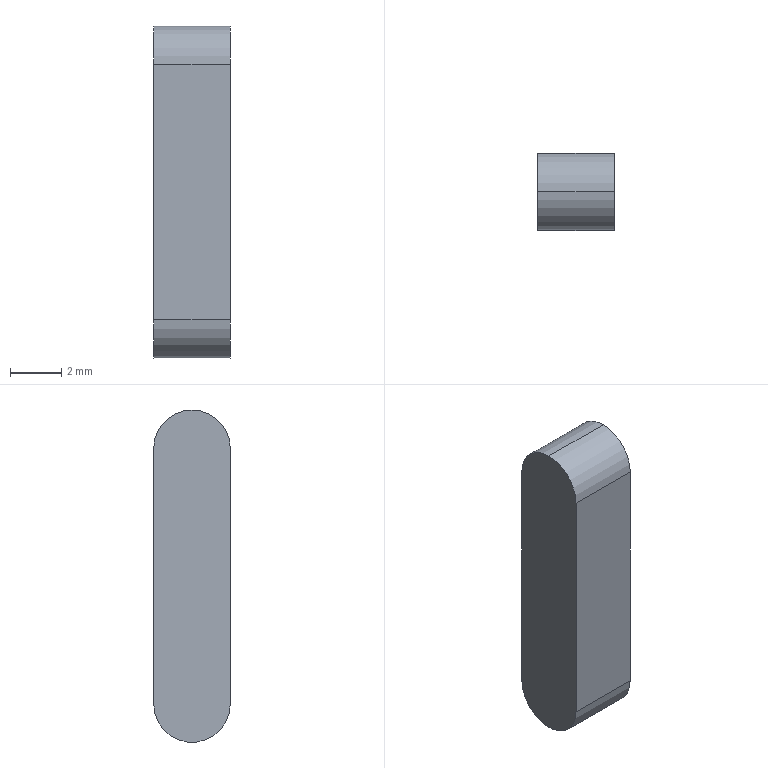Part | STEP file | 06-40 Flat key | 1 solid | 7 faces | box 3 x 3 x 13 mm | volume 111.206 mm3 | plane 4 | cylinder 3 | commonest cylinder face diameters 3 x3
STEP:
#1=CARTESIAN_POINT('',(0.,0.,0.));
#2=DIRECTION('',(0.,0.,1.));
#3=DIRECTION('',(1.,0.,0.));
#4=AXIS2_PLACEMENT_3D('',#1,#2,#3);
#5=CARTESIAN_POINT('',(3.,0.,1.5));
#6=VERTEX_POINT('',#5);
#7=CARTESIAN_POINT('',(3.,-1.5,0.));
#8=VERTEX_POINT('',#7);
#9=CARTESIAN_POINT('',(3.,0.,0.));
#10=DIRECTION('',(1.,0.,0.));
#11=DIRECTION('',(0.,0.,1.));
#12=AXIS2_PLACEMENT_3D('',#9,#10,#11);
#13=CIRCLE('',#12,1.5);
#14=CARTESIAN_POINT('',(3.,0.,0.));
#15=DIRECTION('',(-1.,0.,0.));
#16=DIRECTION('',(0.,0.,1.));
#17=AXIS2_PLACEMENT_3D('',#14,#15,#16);
#18=CYLINDRICAL_SURFACE('',#17,1.5);
#19=CARTESIAN_POINT('',(6.283,0.));
#20=DIRECTION('',(-1.,0.));
#21=VECTOR('',#20,1.);
#22=LINE('',#19,#21);
#23=(GEOMETRIC_REPRESENTATION_CONTEXT(2)PARAMETRIC_REPRESENTATION_CONTEXT()REPRESENTATION_CONTEXT('',''));
#24=DEFINITIONAL_REPRESENTATION('',(#22),#23);
#25=PCURVE('',#18,#24);
#26=CARTESIAN_POINT('',(3.,-1.5,1.578));
#27=DIRECTION('',(1.,0.,0.));
#28=DIRECTION('',(0.,0.,-1.));
#29=AXIS2_PLACEMENT_3D('',#26,#27,#28);
#30=PLANE('',#29);
#31=CARTESIAN_POINT('',(1.578,1.5));
#32=DIRECTION('',(-1.,0.));
#33=AXIS2_PLACEMENT_2D('',#31,#32);
#34=CIRCLE('',#33,1.5);
#35=(GEOMETRIC_REPRESENTATION_CONTEXT(2)PARAMETRIC_REPRESENTATION_CONTEXT()REPRESENTATION_CONTEXT('',''));
#36=DEFINITIONAL_REPRESENTATION('',(#34),#35);
#37=PCURVE('',#30,#36);
#38=SURFACE_CURVE('',#13,(#25,#37),.PCURVE_S1.);
#39=EDGE_CURVE('',#6,#8,#38,.T.);
#40=ORIENTED_EDGE('',*,*,#39,.F.);
#41=CARTESIAN_POINT('',(0.,0.,1.5));
#42=VERTEX_POINT('',#41);
#43=CARTESIAN_POINT('',(3.,0.,1.5));
#44=DIRECTION('',(-1.,0.,0.));
#45=VECTOR('',#44,1.);
#46=LINE('',#43,#45);
#47=CARTESIAN_POINT('',(6.283,0.));
#48=DIRECTION('',(0.,1.));
#49=VECTOR('',#48,1.);
#50=LINE('',#47,#49);
#51=(GEOMETRIC_REPRESENTATION_CONTEXT(2)PARAMETRIC_REPRESENTATION_CONTEXT()REPRESENTATION_CONTEXT('',''));
#52=DEFINITIONAL_REPRESENTATION('',(#50),#51);
#53=PCURVE('',#18,#52);
#54=CARTESIAN_POINT('',(3.,0.,0.));
#55=DIRECTION('',(-1.,0.,0.));
#56=DIRECTION('',(0.,0.,1.));
#57=AXIS2_PLACEMENT_3D('',#54,#55,#56);
#58=CYLINDRICAL_SURFACE('',#57,1.5);
#59=CARTESIAN_POINT('',(0.,0.));
#60=DIRECTION('',(0.,1.));
#61=VECTOR('',#60,1.);
#62=LINE('',#59,#61);
#63=(GEOMETRIC_REPRESENTATION_CONTEXT(2)PARAMETRIC_REPRESENTATION_CONTEXT()REPRESENTATION_CONTEXT('',''));
#64=DEFINITIONAL_REPRESENTATION('',(#62),#63);
#65=PCURVE('',#58,#64);
#66=SURFACE_CURVE('',#46,(#53,#65),.PCURVE_S1.);
#67=EDGE_CURVE('',#6,#42,#66,.T.);
#68=ORIENTED_EDGE('',*,*,#67,.T.);
#69=CARTESIAN_POINT('',(0.,-1.5,0.));
#70=VERTEX_POINT('',#69);
#71=CARTESIAN_POINT('',(0.,0.,0.));
#72=DIRECTION('',(-1.,0.,0.));
#73=DIRECTION('',(0.,0.,1.));
#74=AXIS2_PLACEMENT_3D('',#71,#72,#73);
#75=CIRCLE('',#74,1.5);
#76=CARTESIAN_POINT('',(0.,3.));
#77=DIRECTION('',(1.,0.));
#78=VECTOR('',#77,1.);
#79=LINE('',#76,#78);
#80=(GEOMETRIC_REPRESENTATION_CONTEXT(2)PARAMETRIC_REPRESENTATION_CONTEXT()REPRESENTATION_CONTEXT('',''));
#81=DEFINITIONAL_REPRESENTATION('',(#79),#80);
#82=PCURVE('',#18,#81);
#83=CARTESIAN_POINT('',(0.,-1.5,1.578));
#84=DIRECTION('',(1.,0.,0.));
#85=DIRECTION('',(0.,0.,-1.));
#86=AXIS2_PLACEMENT_3D('',#83,#84,#85);
#87=PLANE('',#86);
#88=CARTESIAN_POINT('',(0.078,1.5));
#89=CARTESIAN_POINT('',(0.078,4.098));
#90=CARTESIAN_POINT('',(2.328,2.799));
#91=CARTESIAN_POINT('',(4.578,1.5));
#92=CARTESIAN_POINT('',(2.328,0.201));
#93=CARTESIAN_POINT('',(0.078,-1.098));
#94=CARTESIAN_POINT('',(0.078,1.5));
#95=(BOUNDED_CURVE()B_SPLINE_CURVE(2,(#88,#89,#90,#91,#92,#93,#94),.UNSPECIFIED.,.T.,.F.)B_SPLINE_CURVE_WITH_KNOTS((1,2,2,2,2,1),(-2.094,0.,2.094,4.189,6.283,8.378),.UNSPECIFIED.)CURVE()GEOMETRIC_REPRESENTATION_ITEM()RATIONAL_B_SPLINE_CURVE((1.,0.5,1.,0.5,1.,0.5,1.))REPRESENTATION_ITEM(''));
#96=(GEOMETRIC_REPRESENTATION_CONTEXT(2)PARAMETRIC_REPRESENTATION_CONTEXT()REPRESENTATION_CONTEXT('',''));
#97=DEFINITIONAL_REPRESENTATION('',(#95),#96);
#98=PCURVE('',#87,#97);
#99=SURFACE_CURVE('',#75,(#82,#98),.PCURVE_S1.);
#100=EDGE_CURVE('',#70,#42,#99,.T.);
#101=ORIENTED_EDGE('',*,*,#100,.F.);
#102=CARTESIAN_POINT('',(1.5,-1.5,-0.000000001));
#103=DIRECTION('',(-1.,0.,0.));
#104=VECTOR('',#103,1.);
#105=LINE('',#102,#104);
#106=CARTESIAN_POINT('',(4.712,1.5));
#107=DIRECTION('',(0.,1.));
#108=VECTOR('',#107,1.);
#109=LINE('',#106,#108);
#110=(GEOMETRIC_REPRESENTATION_CONTEXT(2)PARAMETRIC_REPRESENTATION_CONTEXT()REPRESENTATION_CONTEXT('',''));
#111=DEFINITIONAL_REPRESENTATION('',(#109),#110);
#112=PCURVE('',#18,#111);
#113=CARTESIAN_POINT('',(0.,-1.5,-10.));
#114=DIRECTION('',(0.,1.,0.));
#115=DIRECTION('',(0.,0.,1.));
#116=AXIS2_PLACEMENT_3D('',#113,#114,#115);
#117=PLANE('',#116);
#118=CARTESIAN_POINT('',(10.,1.5));
#119=DIRECTION('',(0.,-1.));
#120=VECTOR('',#119,1.);
#121=LINE('',#118,#120);
#122=(GEOMETRIC_REPRESENTATION_CONTEXT(2)PARAMETRIC_REPRESENTATION_CONTEXT()REPRESENTATION_CONTEXT('',''));
#123=DEFINITIONAL_REPRESENTATION('',(#121),#122);
#124=PCURVE('',#117,#123);
#125=SURFACE_CURVE('',#105,(#112,#124),.PCURVE_S1.);
#126=EDGE_CURVE('',#8,#70,#125,.T.);
#127=ORIENTED_EDGE('',*,*,#126,.F.);
#128=EDGE_LOOP('',(#40,#68,#101,#127));
#129=FACE_BOUND('',#128,.T.);
#130=ADVANCED_FACE('',(#129),#18,.T.);
#131=ORIENTED_EDGE('',*,*,#67,.F.);
#132=CARTESIAN_POINT('',(3.,1.5,0.));
#133=VERTEX_POINT('',#132);
#134=CARTESIAN_POINT('',(3.,0.,0.));
#135=DIRECTION('',(1.,0.,0.));
#136=DIRECTION('',(0.,0.,1.));
#137=AXIS2_PLACEMENT_3D('',#134,#135,#136);
#138=CIRCLE('',#137,1.5);
#139=CARTESIAN_POINT('',(6.283,0.));
#140=DIRECTION('',(-1.,0.));
#141=VECTOR('',#140,1.);
#142=LINE('',#139,#141);
#143=(GEOMETRIC_REPRESENTATION_CONTEXT(2)PARAMETRIC_REPRESENTATION_CONTEXT()REPRESENTATION_CONTEXT('',''));
#144=DEFINITIONAL_REPRESENTATION('',(#142),#143);
#145=PCURVE('',#58,#144);
#146=CARTESIAN_POINT('',(1.578,1.5));
#147=DIRECTION('',(-1.,0.));
#148=AXIS2_PLACEMENT_2D('',#146,#147);
#149=CIRCLE('',#148,1.5);
#150=(GEOMETRIC_REPRESENTATION_CONTEXT(2)PARAMETRIC_REPRESENTATION_CONTEXT()REPRESENTATION_CONTEXT('',''));
#151=DEFINITIONAL_REPRESENTATION('',(#149),#150);
#152=PCURVE('',#30,#151);
#153=SURFACE_CURVE('',#138,(#145,#152),.PCURVE_S1.);
#154=EDGE_CURVE('',#133,#6,#153,.T.);
#155=ORIENTED_EDGE('',*,*,#154,.F.);
#156=CARTESIAN_POINT('',(0.,1.5,0.));
#157=VERTEX_POINT('',#156);
#158=CARTESIAN_POINT('',(1.5,1.5,0.));
#159=DIRECTION('',(1.,0.,0.));
#160=VECTOR('',#159,1.);
#161=LINE('',#158,#160);
#162=CARTESIAN_POINT('',(1.571,1.5));
#163=DIRECTION('',(0.,-1.));
#164=VECTOR('',#163,1.);
#165=LINE('',#162,#164);
#166=(GEOMETRIC_REPRESENTATION_CONTEXT(2)PARAMETRIC_REPRESENTATION_CONTEXT()REPRESENTATION_CONTEXT('',''));
#167=DEFINITIONAL_REPRESENTATION('',(#165),#166);
#168=PCURVE('',#58,#167);
#169=CARTESIAN_POINT('',(0.,1.5,0.));
#170=DIRECTION('',(0.,-1.,0.));
#171=DIRECTION('',(0.,0.,-1.));
#172=AXIS2_PLACEMENT_3D('',#169,#170,#171);
#173=PLANE('',#172);
#174=CARTESIAN_POINT('',(0.,1.5));
#175=DIRECTION('',(0.,1.));
#176=VECTOR('',#175,1.);
#177=LINE('',#174,#176);
#178=(GEOMETRIC_REPRESENTATION_CONTEXT(2)PARAMETRIC_REPRESENTATION_CONTEXT()REPRESENTATION_CONTEXT('',''));
#179=DEFINITIONAL_REPRESENTATION('',(#177),#178);
#180=PCURVE('',#173,#179);
#181=SURFACE_CURVE('',#161,(#168,#180),.PCURVE_S1.);
#182=EDGE_CURVE('',#157,#133,#181,.T.);
#183=ORIENTED_EDGE('',*,*,#182,.F.);
#184=CARTESIAN_POINT('',(0.,0.,0.));
#185=DIRECTION('',(-1.,0.,0.));
#186=DIRECTION('',(0.,0.,1.));
#187=AXIS2_PLACEMENT_3D('',#184,#185,#186);
#188=CIRCLE('',#187,1.5);
#189=CARTESIAN_POINT('',(0.,3.));
#190=DIRECTION('',(1.,0.));
#191=VECTOR('',#190,1.);
#192=LINE('',#189,#191);
#193=(GEOMETRIC_REPRESENTATION_CONTEXT(2)PARAMETRIC_REPRESENTATION_CONTEXT()REPRESENTATION_CONTEXT('',''));
#194=DEFINITIONAL_REPRESENTATION('',(#192),#193);
#195=PCURVE('',#58,#194);
#196=CARTESIAN_POINT('',(0.078,1.5));
#197=CARTESIAN_POINT('',(0.078,4.098));
#198=CARTESIAN_POINT('',(2.328,2.799));
#199=CARTESIAN_POINT('',(4.578,1.5));
#200=CARTESIAN_POINT('',(2.328,0.201));
#201=CARTESIAN_POINT('',(0.078,-1.098));
#202=CARTESIAN_POINT('',(0.078,1.5));
#203=(BOUNDED_CURVE()B_SPLINE_CURVE(2,(#196,#197,#198,#199,#200,#201,#202),.UNSPECIFIED.,.T.,.F.)B_SPLINE_CURVE_WITH_KNOTS((1,2,2,2,2,1),(-2.094,0.,2.094,4.189,6.283,8.378),.UNSPECIFIED.)CURVE()GEOMETRIC_REPRESENTATION_ITEM()RATIONAL_B_SPLINE_CURVE((1.,0.5,1.,0.5,1.,0.5,1.))REPRESENTATION_ITEM(''));
#204=(GEOMETRIC_REPRESENTATION_CONTEXT(2)PARAMETRIC_REPRESENTATION_CONTEXT()REPRESENTATION_CONTEXT('',''));
#205=DEFINITIONAL_REPRESENTATION('',(#203),#204);
#206=PCURVE('',#87,#205);
#207=SURFACE_CURVE('',#188,(#195,#206),.PCURVE_S1.);
#208=EDGE_CURVE('',#42,#157,#207,.T.);
#209=ORIENTED_EDGE('',*,*,#208,.F.);
#210=EDGE_LOOP('',(#131,#155,#183,#209));
#211=FACE_BOUND('',#210,.T.);
#212=ADVANCED_FACE('',(#211),#58,.T.);
#213=CARTESIAN_POINT('',(3.,-1.5,-10.));
#214=VERTEX_POINT('',#213);
#215=CARTESIAN_POINT('',(3.,1.5,-10.));
#216=VERTEX_POINT('',#215);
#217=CARTESIAN_POINT('',(3.,0.,-10.));
#218=DIRECTION('',(1.,0.,0.));
#219=DIRECTION('',(0.,0.,1.));
#220=AXIS2_PLACEMENT_3D('',#217,#218,#219);
#221=CIRCLE('',#220,1.5);
#222=CARTESIAN_POINT('',(11.578,1.5));
#223=DIRECTION('',(-1.,0.));
#224=AXIS2_PLACEMENT_2D('',#222,#223);
#225=CIRCLE('',#224,1.5);
#226=(GEOMETRIC_REPRESENTATION_CONTEXT(2)PARAMETRIC_REPRESENTATION_CONTEXT()REPRESENTATION_CONTEXT('',''));
#227=DEFINITIONAL_REPRESENTATION('',(#225),#226);
#228=PCURVE('',#30,#227);
#229=CARTESIAN_POINT('',(3.,0.,-10.));
#230=DIRECTION('',(-1.,0.,0.));
#231=DIRECTION('',(0.,0.,1.));
#232=AXIS2_PLACEMENT_3D('',#229,#230,#231);
#233=CYLINDRICAL_SURFACE('',#232,1.5);
#234=CARTESIAN_POINT('',(6.283,0.));
#235=DIRECTION('',(-1.,0.));
#236=VECTOR('',#235,1.);
#237=LINE('',#234,#236);
#238=(GEOMETRIC_REPRESENTATION_CONTEXT(2)PARAMETRIC_REPRESENTATION_CONTEXT()REPRESENTATION_CONTEXT('',''));
#239=DEFINITIONAL_REPRESENTATION('',(#237),#238);
#240=PCURVE('',#233,#239);
#241=SURFACE_CURVE('',#221,(#228,#240),.PCURVE_S1.);
#242=EDGE_CURVE('',#214,#216,#241,.T.);
#243=ORIENTED_EDGE('',*,*,#242,.T.);
#244=CARTESIAN_POINT('',(3.,1.5,-5.));
#245=DIRECTION('',(0.,0.,1.));
#246=VECTOR('',#245,1.);
#247=LINE('',#244,#246);
#248=CARTESIAN_POINT('',(6.578,3.));
#249=DIRECTION('',(-1.,0.));
#250=VECTOR('',#249,1.);
#251=LINE('',#248,#250);
#252=(GEOMETRIC_REPRESENTATION_CONTEXT(2)PARAMETRIC_REPRESENTATION_CONTEXT()REPRESENTATION_CONTEXT('',''));
#253=DEFINITIONAL_REPRESENTATION('',(#251),#252);
#254=PCURVE('',#30,#253);
#255=CARTESIAN_POINT('',(5.,3.));
#256=DIRECTION('',(-1.,0.));
#257=VECTOR('',#256,1.);
#258=LINE('',#255,#257);
#259=(GEOMETRIC_REPRESENTATION_CONTEXT(2)PARAMETRIC_REPRESENTATION_CONTEXT()REPRESENTATION_CONTEXT('',''));
#260=DEFINITIONAL_REPRESENTATION('',(#258),#259);
#261=PCURVE('',#173,#260);
#262=SURFACE_CURVE('',#247,(#254,#261),.PCURVE_S1.);
#263=EDGE_CURVE('',#216,#133,#262,.T.);
#264=ORIENTED_EDGE('',*,*,#263,.T.);
#265=ORIENTED_EDGE('',*,*,#154,.T.);
#266=ORIENTED_EDGE('',*,*,#39,.T.);
#267=CARTESIAN_POINT('',(3.,-1.5,-5.));
#268=DIRECTION('',(0.,0.,-1.));
#269=VECTOR('',#268,1.);
#270=LINE('',#267,#269);
#271=CARTESIAN_POINT('',(6.578,0.));
#272=DIRECTION('',(1.,0.));
#273=VECTOR('',#272,1.);
#274=LINE('',#271,#273);
#275=(GEOMETRIC_REPRESENTATION_CONTEXT(2)PARAMETRIC_REPRESENTATION_CONTEXT()REPRESENTATION_CONTEXT('',''));
#276=DEFINITIONAL_REPRESENTATION('',(#274),#275);
#277=PCURVE('',#30,#276);
#278=CARTESIAN_POINT('',(5.,3.));
#279=DIRECTION('',(-1.,0.));
#280=VECTOR('',#279,1.);
#281=LINE('',#278,#280);
#282=(GEOMETRIC_REPRESENTATION_CONTEXT(2)PARAMETRIC_REPRESENTATION_CONTEXT()REPRESENTATION_CONTEXT('',''));
#283=DEFINITIONAL_REPRESENTATION('',(#281),#282);
#284=PCURVE('',#117,#283);
#285=SURFACE_CURVE('',#270,(#277,#284),.PCURVE_S1.);
#286=EDGE_CURVE('',#8,#214,#285,.T.);
#287=ORIENTED_EDGE('',*,*,#286,.T.);
#288=EDGE_LOOP('',(#243,#264,#265,#266,#287));
#289=FACE_BOUND('',#288,.T.);
#290=ADVANCED_FACE('',(#289),#30,.T.);
#291=CARTESIAN_POINT('',(0.,1.5,-10.));
#292=VERTEX_POINT('',#291);
#293=CARTESIAN_POINT('',(0.,1.5,-5.));
#294=DIRECTION('',(0.,0.,1.));
#295=VECTOR('',#294,1.);
#296=LINE('',#293,#295);
#297=CARTESIAN_POINT('',(6.578,3.));
#298=DIRECTION('',(-1.,0.));
#299=VECTOR('',#298,1.);
#300=LINE('',#297,#299);
#301=(GEOMETRIC_REPRESENTATION_CONTEXT(2)PARAMETRIC_REPRESENTATION_CONTEXT()REPRESENTATION_CONTEXT('',''));
#302=DEFINITIONAL_REPRESENTATION('',(#300),#301);
#303=PCURVE('',#87,#302);
#304=CARTESIAN_POINT('',(5.,0.));
#305=DIRECTION('',(-1.,0.));
#306=VECTOR('',#305,1.);
#307=LINE('',#304,#306);
#308=(GEOMETRIC_REPRESENTATION_CONTEXT(2)PARAMETRIC_REPRESENTATION_CONTEXT()REPRESENTATION_CONTEXT('',''));
#309=DEFINITIONAL_REPRESENTATION('',(#307),#308);
#310=PCURVE('',#173,#309);
#311=SURFACE_CURVE('',#296,(#303,#310),.PCURVE_S1.);
#312=EDGE_CURVE('',#292,#157,#311,.T.);
#313=ORIENTED_EDGE('',*,*,#312,.F.);
#314=CARTESIAN_POINT('',(0.,-1.5,-10.));
#315=VERTEX_POINT('',#314);
#316=CARTESIAN_POINT('',(0.,0.,-10.));
#317=DIRECTION('',(1.,0.,0.));
#318=DIRECTION('',(0.,0.,1.));
#319=AXIS2_PLACEMENT_3D('',#316,#317,#318);
#320=CIRCLE('',#319,1.5);
#321=CARTESIAN_POINT('',(11.578,1.5));
#322=DIRECTION('',(-1.,0.));
#323=AXIS2_PLACEMENT_2D('',#321,#322);
#324=CIRCLE('',#323,1.5);
#325=(GEOMETRIC_REPRESENTATION_CONTEXT(2)PARAMETRIC_REPRESENTATION_CONTEXT()REPRESENTATION_CONTEXT('',''));
#326=DEFINITIONAL_REPRESENTATION('',(#324),#325);
#327=PCURVE('',#87,#326);
#328=CARTESIAN_POINT('',(6.283,3.));
#329=DIRECTION('',(-1.,0.));
#330=VECTOR('',#329,1.);
#331=LINE('',#328,#330);
#332=(GEOMETRIC_REPRESENTATION_CONTEXT(2)PARAMETRIC_REPRESENTATION_CONTEXT()REPRESENTATION_CONTEXT('',''));
#333=DEFINITIONAL_REPRESENTATION('',(#331),#332);
#334=PCURVE('',#233,#333);
#335=SURFACE_CURVE('',#320,(#327,#334),.PCURVE_S1.);
#336=EDGE_CURVE('',#315,#292,#335,.T.);
#337=ORIENTED_EDGE('',*,*,#336,.F.);
#338=CARTESIAN_POINT('',(0.,-1.5,-5.));
#339=DIRECTION('',(0.,0.,-1.));
#340=VECTOR('',#339,1.);
#341=LINE('',#338,#340);
#342=CARTESIAN_POINT('',(6.578,0.));
#343=DIRECTION('',(1.,0.));
#344=VECTOR('',#343,1.);
#345=LINE('',#342,#344);
#346=(GEOMETRIC_REPRESENTATION_CONTEXT(2)PARAMETRIC_REPRESENTATION_CONTEXT()REPRESENTATION_CONTEXT('',''));
#347=DEFINITIONAL_REPRESENTATION('',(#345),#346);
#348=PCURVE('',#87,#347);
#349=CARTESIAN_POINT('',(5.,0.));
#350=DIRECTION('',(-1.,0.));
#351=VECTOR('',#350,1.);
#352=LINE('',#349,#351);
#353=(GEOMETRIC_REPRESENTATION_CONTEXT(2)PARAMETRIC_REPRESENTATION_CONTEXT()REPRESENTATION_CONTEXT('',''));
#354=DEFINITIONAL_REPRESENTATION('',(#352),#353);
#355=PCURVE('',#117,#354);
#356=SURFACE_CURVE('',#341,(#348,#355),.PCURVE_S1.);
#357=EDGE_CURVE('',#70,#315,#356,.T.);
#358=ORIENTED_EDGE('',*,*,#357,.F.);
#359=ORIENTED_EDGE('',*,*,#100,.T.);
#360=ORIENTED_EDGE('',*,*,#208,.T.);
#361=EDGE_LOOP('',(#313,#337,#358,#359,#360));
#362=FACE_BOUND('',#361,.T.);
#363=ADVANCED_FACE('',(#362),#87,.F.);
#364=CARTESIAN_POINT('',(1.5,-1.5,-10.));
#365=DIRECTION('',(-1.,0.,0.));
#366=VECTOR('',#365,1.);
#367=LINE('',#364,#366);
#368=CARTESIAN_POINT('',(0.,1.5));
#369=DIRECTION('',(0.,-1.));
#370=VECTOR('',#369,1.);
#371=LINE('',#368,#370);
#372=(GEOMETRIC_REPRESENTATION_CONTEXT(2)PARAMETRIC_REPRESENTATION_CONTEXT()REPRESENTATION_CONTEXT('',''));
#373=DEFINITIONAL_REPRESENTATION('',(#371),#372);
#374=PCURVE('',#117,#373);
#375=CARTESIAN_POINT('',(4.712,1.5));
#376=DIRECTION('',(0.,1.));
#377=VECTOR('',#376,1.);
#378=LINE('',#375,#377);
#379=(GEOMETRIC_REPRESENTATION_CONTEXT(2)PARAMETRIC_REPRESENTATION_CONTEXT()REPRESENTATION_CONTEXT('',''));
#380=DEFINITIONAL_REPRESENTATION('',(#378),#379);
#381=PCURVE('',#233,#380);
#382=SURFACE_CURVE('',#367,(#374,#381),.PCURVE_S1.);
#383=EDGE_CURVE('',#214,#315,#382,.T.);
#384=ORIENTED_EDGE('',*,*,#383,.F.);
#385=ORIENTED_EDGE('',*,*,#286,.F.);
#386=ORIENTED_EDGE('',*,*,#126,.T.);
#387=ORIENTED_EDGE('',*,*,#357,.T.);
#388=EDGE_LOOP('',(#384,#385,#386,#387));
#389=FACE_BOUND('',#388,.T.);
#390=ADVANCED_FACE('',(#389),#117,.F.);
#391=ORIENTED_EDGE('',*,*,#182,.T.);
#392=ORIENTED_EDGE('',*,*,#263,.F.);
#393=CARTESIAN_POINT('',(1.5,1.5,-10.));
#394=DIRECTION('',(1.,0.,0.));
#395=VECTOR('',#394,1.);
#396=LINE('',#393,#395);
#397=CARTESIAN_POINT('',(10.,1.5));
#398=DIRECTION('',(0.,1.));
#399=VECTOR('',#398,1.);
#400=LINE('',#397,#399);
#401=(GEOMETRIC_REPRESENTATION_CONTEXT(2)PARAMETRIC_REPRESENTATION_CONTEXT()REPRESENTATION_CONTEXT('',''));
#402=DEFINITIONAL_REPRESENTATION('',(#400),#401);
#403=PCURVE('',#173,#402);
#404=CARTESIAN_POINT('',(1.571,1.5));
#405=DIRECTION('',(0.,-1.));
#406=VECTOR('',#405,1.);
#407=LINE('',#404,#406);
#408=(GEOMETRIC_REPRESENTATION_CONTEXT(2)PARAMETRIC_REPRESENTATION_CONTEXT()REPRESENTATION_CONTEXT('',''));
#409=DEFINITIONAL_REPRESENTATION('',(#407),#408);
#410=PCURVE('',#233,#409);
#411=SURFACE_CURVE('',#396,(#403,#410),.PCURVE_S1.);
#412=EDGE_CURVE('',#292,#216,#411,.T.);
#413=ORIENTED_EDGE('',*,*,#412,.F.);
#414=ORIENTED_EDGE('',*,*,#312,.T.);
#415=EDGE_LOOP('',(#391,#392,#413,#414));
#416=FACE_BOUND('',#415,.T.);
#417=ADVANCED_FACE('',(#416),#173,.F.);
#418=ORIENTED_EDGE('',*,*,#412,.T.);
#419=ORIENTED_EDGE('',*,*,#242,.F.);
#420=ORIENTED_EDGE('',*,*,#383,.T.);
#421=ORIENTED_EDGE('',*,*,#336,.T.);
#422=EDGE_LOOP('',(#418,#419,#420,#421));
#423=FACE_BOUND('',#422,.T.);
#424=ADVANCED_FACE('',(#423),#233,.T.);
#425=CLOSED_SHELL('',(#130,#212,#290,#363,#390,#417,#424));
#426=MANIFOLD_SOLID_BREP('',#425);
#427=(LENGTH_UNIT()NAMED_UNIT(*)SI_UNIT(.MILLI.,.METRE.));
#428=UNCERTAINTY_MEASURE_WITH_UNIT(LENGTH_MEASURE(0.0000001),#427,'','');
#429=(NAMED_UNIT(*)PLANE_ANGLE_UNIT()SI_UNIT($,.RADIAN.));
#430=(NAMED_UNIT(*)SI_UNIT($,.STERADIAN.)SOLID_ANGLE_UNIT());
#431=(GEOMETRIC_REPRESENTATION_CONTEXT(3)GLOBAL_UNCERTAINTY_ASSIGNED_CONTEXT((#428))GLOBAL_UNIT_ASSIGNED_CONTEXT((#427,#429,#430))REPRESENTATION_CONTEXT('',''));
#432=ADVANCED_BREP_SHAPE_REPRESENTATION('',(#4,#426),#431);